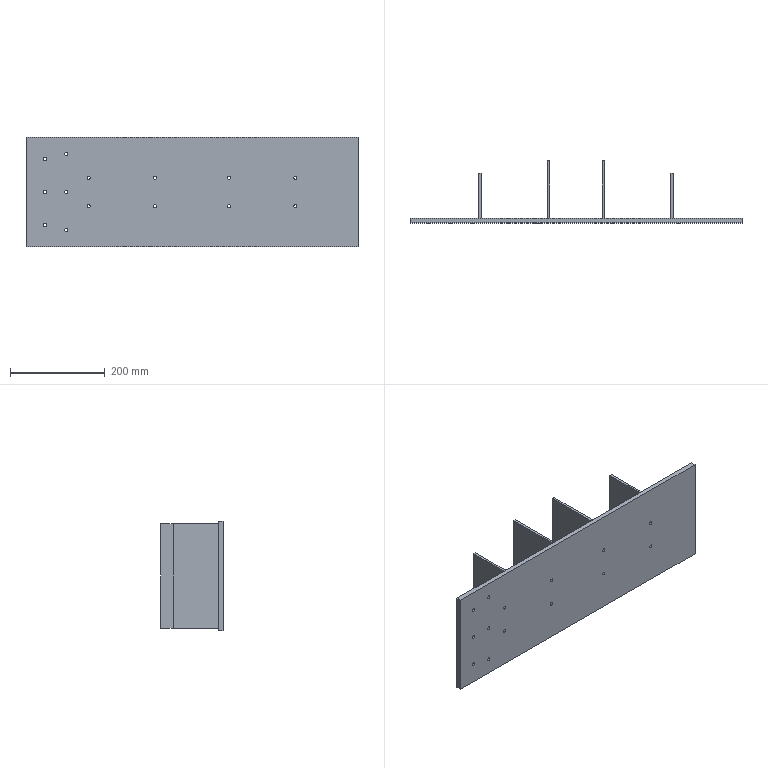Part | SolidWorks | features HoleWzd 3, ICE 2, Extrusion 1 | 1 solid | 54 faces | box 700 x 131 x 230 mm | volume 2080116 mm3 | cylinder 28 | plane 26 | commonest cylinder face diameters 6.8 x28